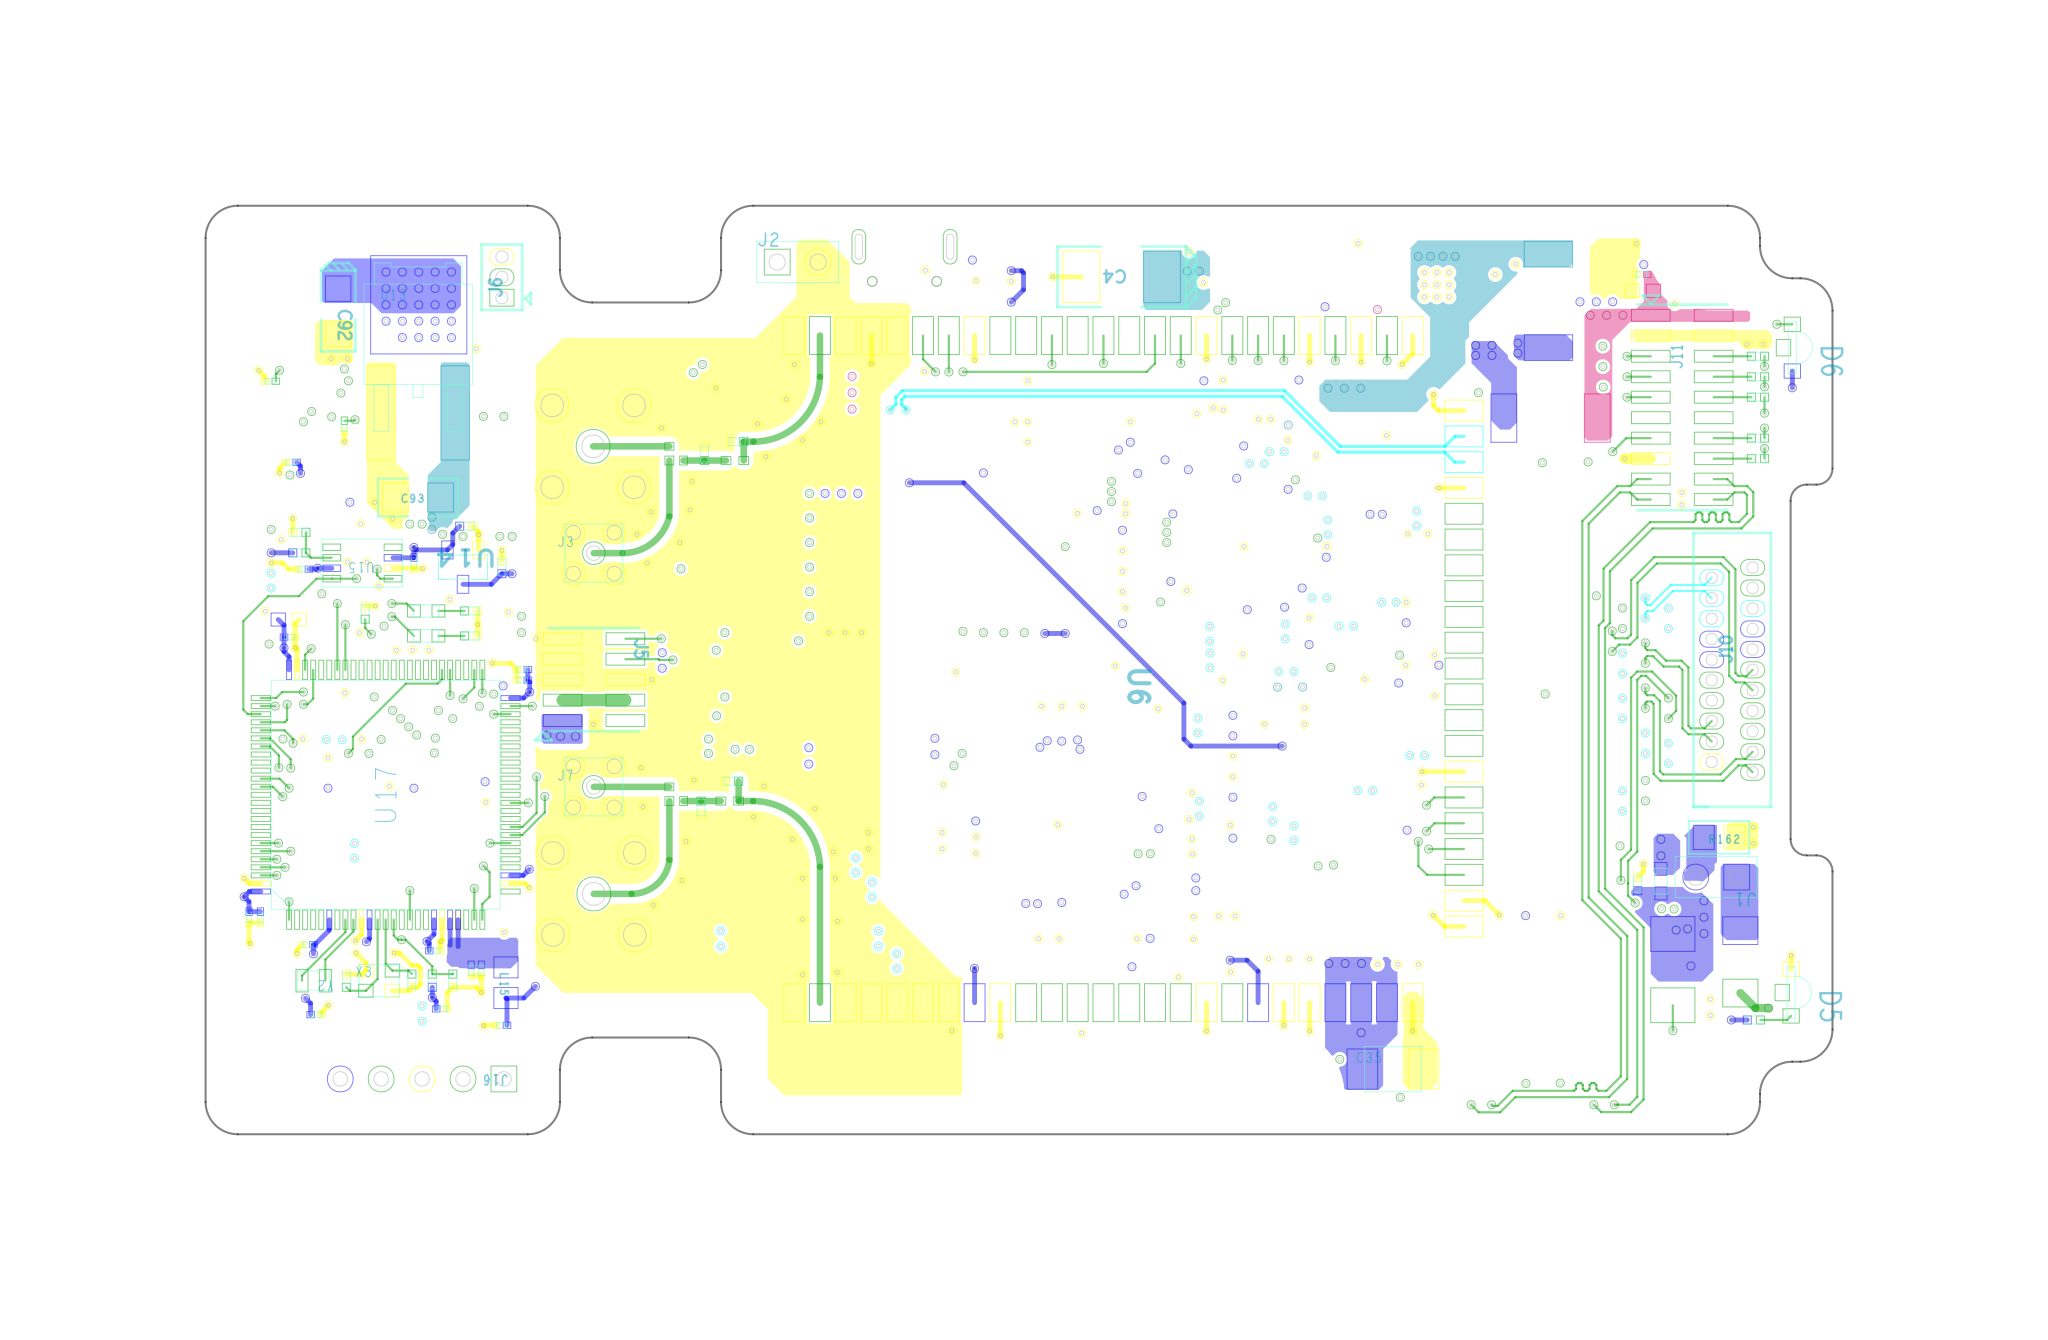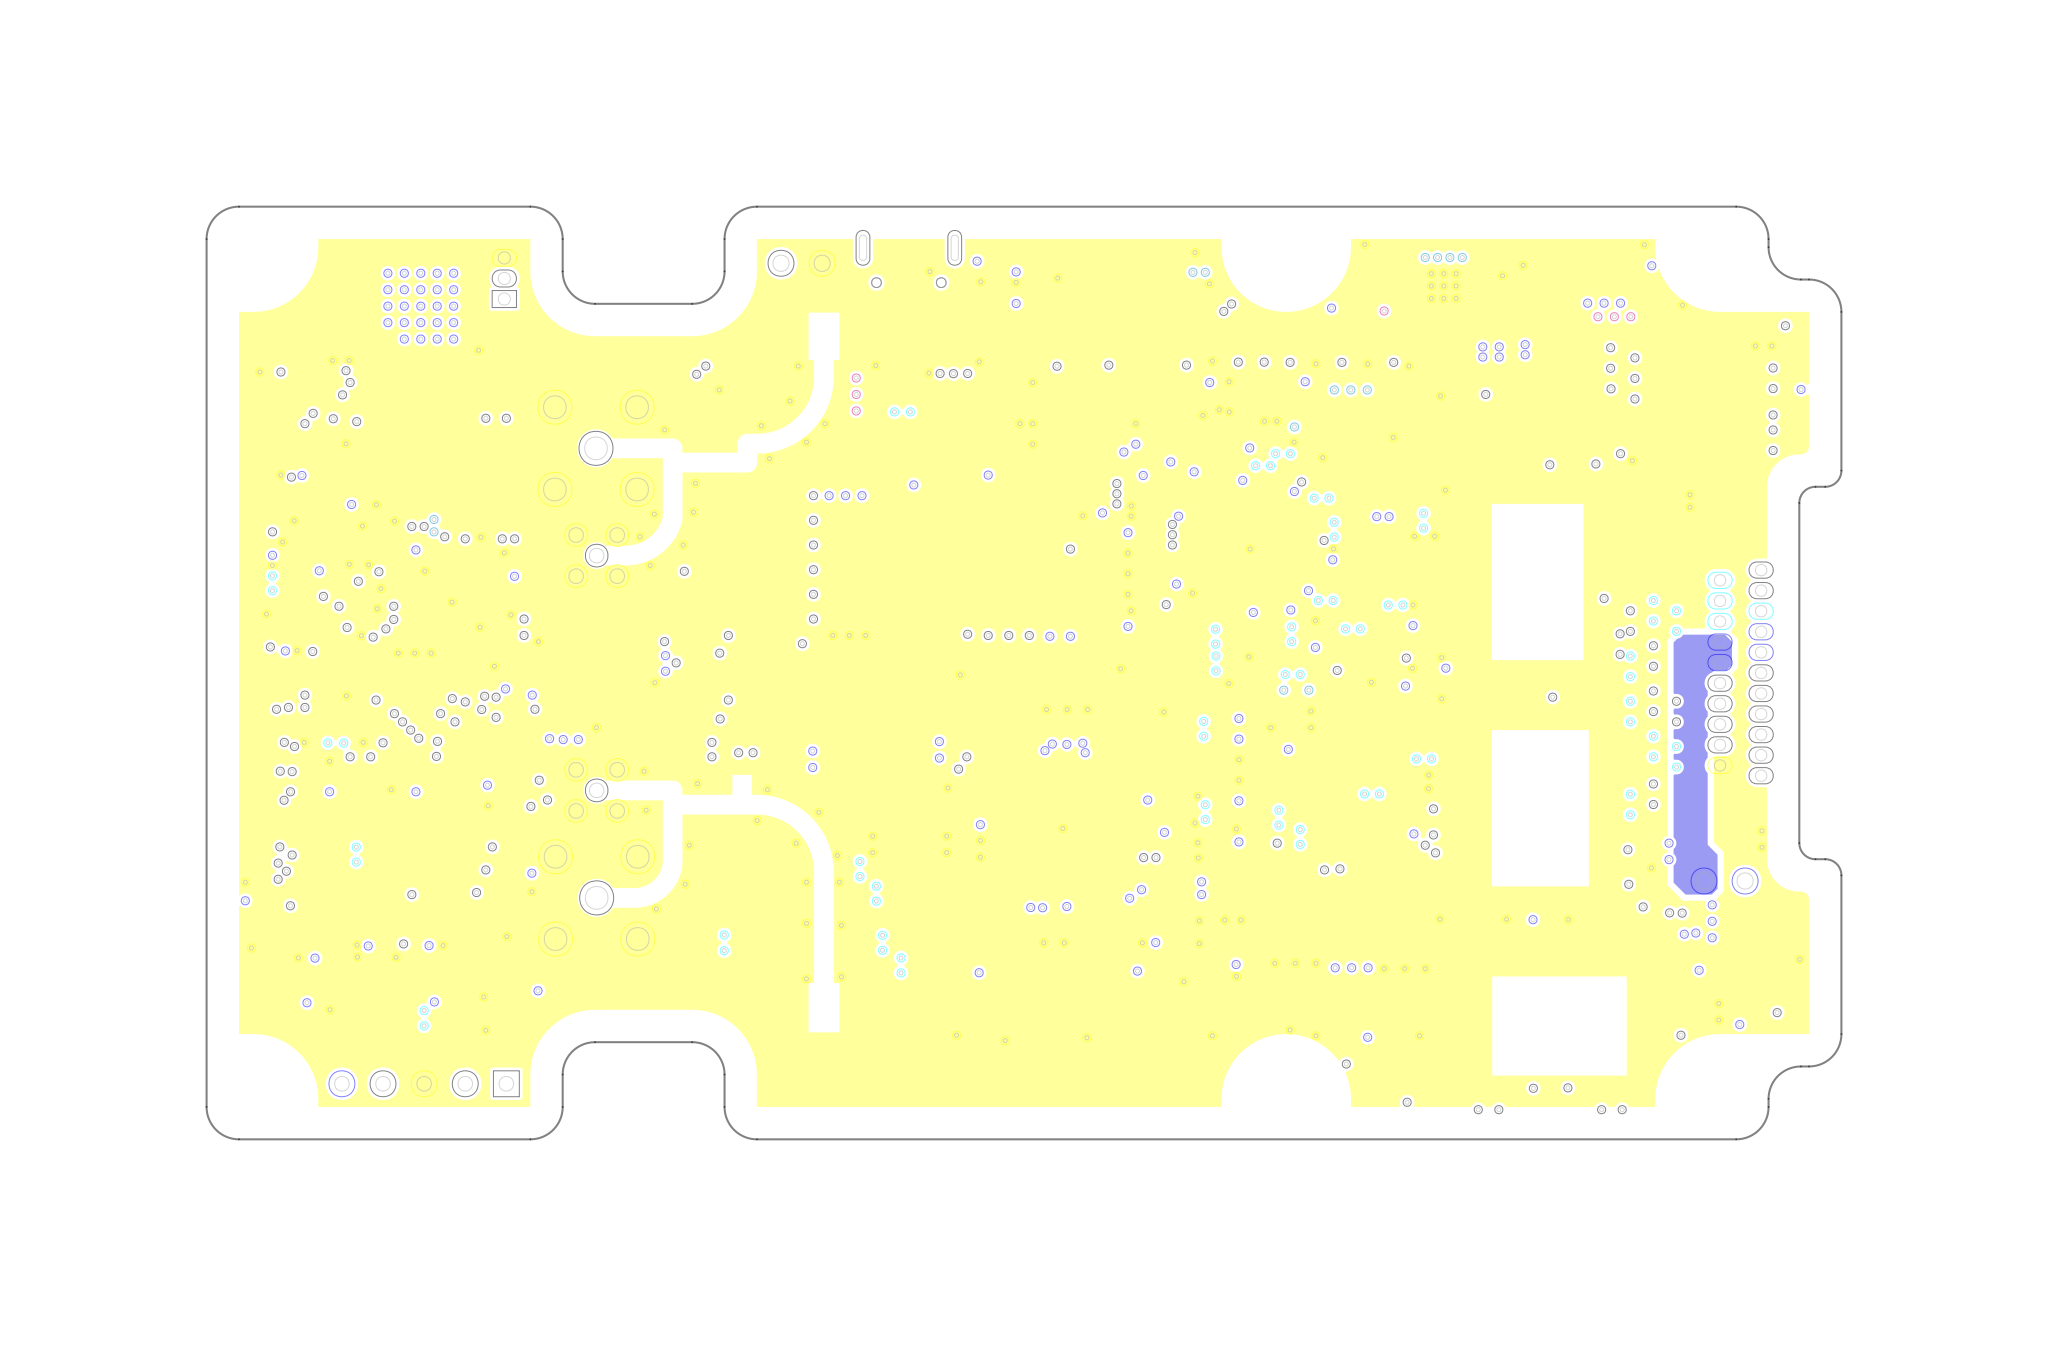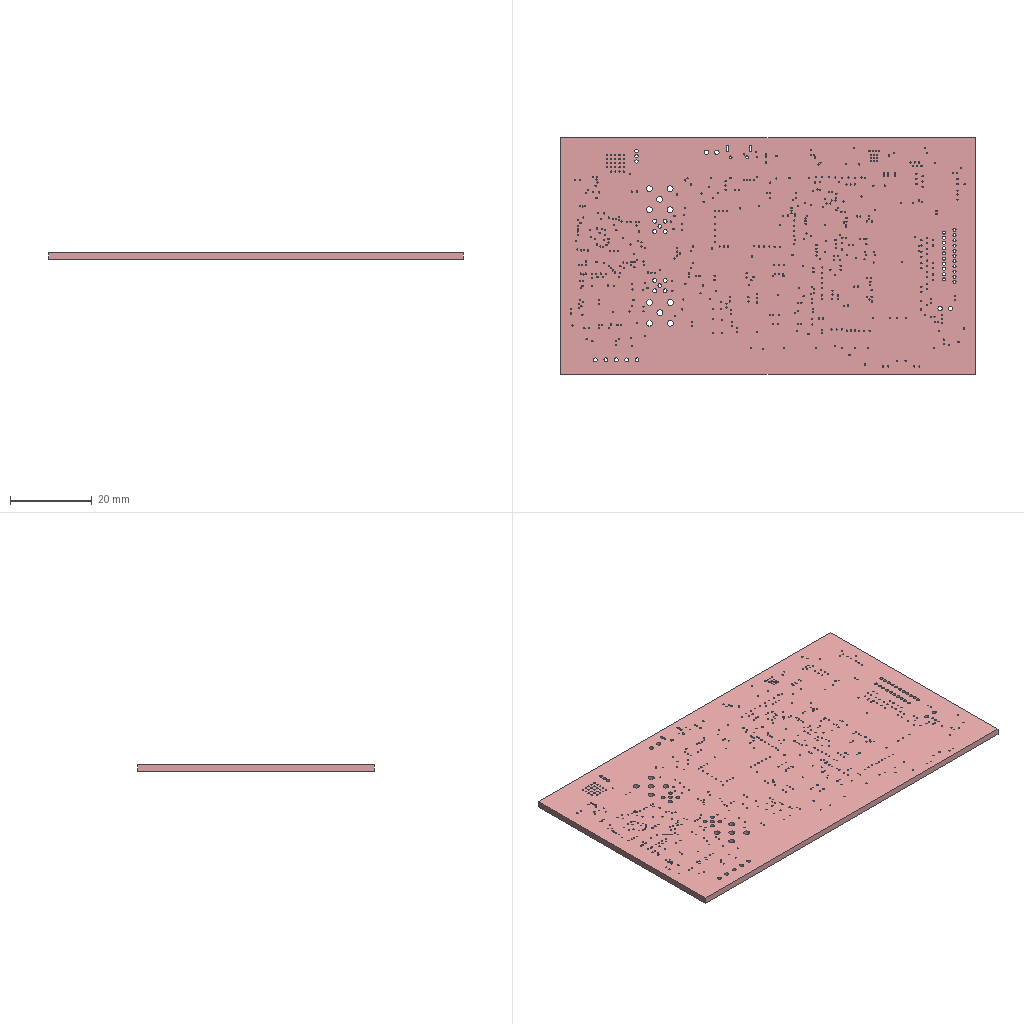Circuit board layout | Cadence Allegro | box 101.1 x 57.7 x 1.6 mm
Layer stack:
# Cadence Allegro layer stack of  (unit mm; from the constraint file cross-section; dielectric type: 0 not recorded (Allegro does not mark core vs prepreg), 3 surface material)
index,name,kind,layer,copper_thickness_mm,dielectric_type,dielectric_thickness_mm,dielectric_material,dielectric_constant
0,Top Surface,other,,,,,,
1,TOP,copper,TOP,0.0305,,,,
2,Dielectric1,dielectric,,,0,0.2032,FR-4,4.5
3,L2_GND,copper,L2_GND,0.0305,,,,
4,Dielectric2,dielectric,,,0,0.2032,FR-4,4.5
5,L3_S1,copper,L3_S1,0.0305,,,,
6,Dielectric3,dielectric,,,0,0.2032,FR-4,4.5
7,L4_PWR,copper,L4_PWR,0.0305,,,,
8,Dielectric4,dielectric,,,0,0.2032,FR-4,4.5
9,L5_GND,copper,L5_GND,0.0305,,,,
10,Dielectric5,dielectric,,,0,0.2032,FR-4,4.5
11,L6_S2,copper,L6_S2,0.0305,,,,
12,Dielectric6,dielectric,,,0,0.2032,FR-4,4.5
13,L7_GND,copper,L7_GND,0.0305,,,,
14,Dielectric7,dielectric,,,0,0.2032,FR-4,4.5
15,BOTTOM,copper,BOTTOM,0.0305,,,,
16,Bottom Surface,other,,,,,,
# drill layer pairs: low layer,high layer
drill_pair,TOP,BOTTOM
Part placement:
REFDES,COMP_VALUE,SYM_NAME,SYM_X,SYM_Y,SYM_ROTATE,SYM_MIRROR
C1,0.1uF,50V,0402C,3556.000,1461.000,270.000,NO
C2,4.7uF,50V,0805C,3075.000,2768.000,0.000,YES
C3,100uF,16V,C,CA45C,3630.000,2577.000,90.000,YES
C4,100uF,16V,C,CA45C,2295.000,2944.000,180.000,NO
C5,4.7uF,50V,0805C,2880.000,2411.000,0.000,YES
C6,4.7uF,50V,0805C,3649.000,1260.000,90.000,YES
C7,4.7uF,50V,0805C,3734.000,1260.000,90.000,YES
C8,4.7uF,50V,0805C,3507.000,2962.000,270.000,YES
C9,4.7uF,50V,0805C,3417.000,2962.000,270.000,YES
C10,0.1uF,50V,0402C,3338.000,2972.000,270.000,YES
C11,4.7uF,50V,0805C,3185.000,2527.000,270.000,YES
C12,4.7uF,50V,0805C,3270.000,2527.000,270.000,YES
C13,0.1uF,50V,0402C,3115.000,2552.000,270.000,YES
C14,0.1uF,50V,0402C,3249.000,3001.000,180.000,YES
C15,82pF,50V,0402C,2745.000,2582.000,0.000,YES
C16,22uF,10V,0603C,2704.000,1915.000,90.000,YES
C17,2.2uF,10V,0402C,2767.000,1928.000,90.000,YES
C18,82pF,50V,0402C,2889.000,2892.000,0.000,YES
C19,22uF,10V,0603C,2645.000,1914.000,90.000,YES
C20,0.1uF,50V,0402C,3658.000,1131.000,180.000,YES
C21,22uF,10V,0603C,2709.000,1220.000,270.000,YES
C22,22uF,10V,0603C,2654.000,1220.000,270.000,YES
C23,22uF,10V,0603C,2764.000,1220.000,270.000,YES
C24,22uF,10V,0603C,2599.000,1220.000,270.000,YES
C25,330uF,6.3V,C,CA45C,2734.000,1360.000,0.000,YES
C26,0.1uF,50V,0402C,3130.000,2632.000,180.000,YES
C27,0.1uF,10V,0402C,3019.000,2021.000,180.000,YES
C28,0.1uF,10V,0402C,2405.000,2980.000,0.000,YES
C29,0.1uF,10V,0402C,1980.000,2935.000,180.000,YES
C30,0.1uF,10V,0402C,2405.000,2880.000,0.000,YES
C31,0.1uF,10V(NC),0402C,2574.000,2688.000,270.000,YES
C32,0.1uF,10V,0402C,2405.000,2930.000,0.000,YES
C33,0.1uF,10V,0402C,2405.000,2830.000,0.000,YES
C34,0.1uF,10V,0402C,2904.000,1235.000,180.000,YES
C35,47uF,10V,B,CAKB,2958.000,1009.000,0.000,NO
C36,1pF,200V,0402C,1275.000,2511.492,90.000,NO
C37,1pF,200V,0402C,1355.000,2541.350,180.000,NO
C38,1pF,200V,0402C,1267.000,1647.547,270.000,NO
C39,1pF,200V,0402C,1342.512,1712.000,180.000,NO
C40,10pF,50V,0402C,2526.000,1923.000,180.000,YES
C41,10pF,50V,0402C,2526.000,1773.000,180.000,YES
C42,0.1uF,10V,0402C,2092.000,1371.000,90.000,YES
C43,0.1uF,10V,0402C,2099.000,1853.000,270.000,YES
C44,0.1uF,10V,0402C,2427.000,1326.000,180.000,YES
C45,0.1uF,10V,0402C,2199.000,1853.000,270.000,YES
C46,0.1uF,10V,0402C,1902.000,1595.000,90.000,YES
C47,10pF,50V,0402C,2526.000,1623.000,180.000,YES
C48,10pF,50V,0402C,2526.000,1723.000,180.000,YES
C49,1uF,25V,0402C,2427.000,1571.000,180.000,YES
C50,0.1uF,10V,0402C,2386.000,1224.000,180.000,YES
C51,0.1uF,10V,0402C,2332.000,1371.000,90.000,YES
C52,0.1uF,10V,0402C,2427.000,1684.000,180.000,YES
C53,27pF,50V,0402C,2197.000,1174.000,90.000,YES
C54,27pF,50V,0402C,1880.000,1173.000,90.000,YES
C55,1uF,25V,0402C,2142.000,1371.000,90.000,YES
C56,0.1uF,10V,0402C,2293.000,1275.000,270.000,YES
C57,0.1uF,10V,0402C,2149.000,1853.000,270.000,YES
C58,0.1uF,10V,0402C,2427.000,1521.000,180.000,YES
C59,0.1uF,10V,0402C,2427.000,1381.000,180.000,YES
C60,1uF,25V,0402C,2218.000,1356.000,180.000,YES
C61,0.1uF,10V,0402C,2218.000,1308.000,180.000,YES
C62,22pF,16V,0402C,2340.000,1889.000,180.000,YES
C63,22pF,16V,0402C,2340.000,2049.000,0.000,YES
C64,22uF,10V,0603C,2261.000,2303.000,270.000,YES
C65,0.1uF,25V,0201C,1859.000,1761.000,90.000,YES
C66,47uF,16V,C,CA45C,1759.000,1676.000,90.000,YES
C67,47uF,16V,C,CA45C,1470.000,2672.000,0.000,YES
C68,4.7uF,16V,0603C,3569.000,2910.000,0.000,NO
C69,0.1uF,25V,0201C,3566.000,2950.000,180.000,NO
C70,0.1uF,25V,0201C,3325.000,1364.000,90.000,YES
C71,0.1uF,25V,0201C,2819.000,2272.000,90.000,YES
C72,0.1uF,25V,0201C,2603.000,2090.000,270.000,YES
C73,0.1uF,25V,0201C,2736.000,2134.000,0.000,YES
C74,0.1uF,25V,0201C,2757.000,2433.000,0.000,YES
C77,0.1uF,25V,0201C,2659.000,2558.000,90.000,YES
C78,0.1uF,25V,0201C,2454.000,2573.000,90.000,YES
C79,4.7uF,16V,0603C,2574.000,2593.000,90.000,YES
C80,NC,0402C,2519.000,2583.000,90.000,YES
C81,0.1uF,25V,0201C,2629.000,2558.000,90.000,YES
C82,0.1uF,25V,0201C,2479.000,2573.000,90.000,YES
C83,0.022uF,25V,0402C,3384.000,1359.000,0.000,YES
C84,0.01uF,2KV,1812C,2975.000,1075.000,270.000,YES
C85,0.1uF,25V,0201C,2343.000,2365.000,0.000,YES
C86,0.1uF,25V,0201C,2343.000,2135.000,0.000,YES
C87,0.022uF,25V,0402C,3031.000,2149.000,0.000,YES
C88,0.01uF,2KV,1812C,2865.000,1715.000,0.000,YES
C89,0.1uF,25V,0201C,2343.000,2390.000,0.000,YES
C90,22uF,10V,0603C,2187.000,2422.000,270.000,YES
C91,47uF,16V,C,CA45C,1618.000,2240.000,90.000,YES
C92,10uF,16V,A,CA45A,380.000,2860.000,270.000,NO
C93,10uF,25V,1206C,575.000,2405.000,0.000,NO
C94,0.1uF,25V,0201C,565.000,2245.000,270.000,NO
C95,0.1uF,25V,0201C,295.000,2230.000,180.000,NO
C96,1uF,25V,0402C,780.000,2235.000,270.000,NO
C97,NC,0402C,437.000,1857.000,270.000,YES
C98,NC,0402C,293.000,1857.000,270.000,YES
C99,NC,0402C,257.000,2127.000,180.000,YES
C100,NC,0402C,257.000,2277.000,180.000,YES
C101,1uF,25V,0402C,693.000,2335.000,180.000,NO
C102,0.1uF,25V,0201C,715.000,2000.000,180.000,YES
C103,0.1uF,25V,0201C,446.000,2099.000,0.000,YES
C104,0.1uF,25V,0201C,430.000,1919.000,0.000,YES
C105,0.1uF,25V,0201C,956.000,2062.000,90.000,YES
C106,10uF,25V,1206C,1019.000,2040.000,270.000,YES
C107,22pF,16V,0402C,505.000,2205.000,90.000,YES
C108,0.1uF,25V,0201C,755.000,2125.000,180.000,YES
C109,10uF,25V,1206C,810.000,2200.000,0.000,YES
C110,22pF,16V,0402C,665.000,2205.000,270.000,YES
C111,0.1uF,25V,0201C,817.000,1476.000,90.000,YES
C112,2.2uF,25V,0603C,925.000,1896.000,0.000,YES
C113,2.2uF,25V,0603C,291.000,1997.000,180.000,YES
C114,22pF,16V,0402C,400.000,1225.000,90.000,NO
C115,4.7uF,16V,0603C,259.000,2107.000,180.000,NO
C116,0.1uF,25V,0201C,790.000,1476.000,90.000,YES
C117,0.1uF,25V,0201C,162.000,1380.000,270.000,NO
C118,0.1uF,25V,0201C,616.000,1298.000,0.000,NO
C119,0.1uF,25V,0201C,190.000,1380.000,270.000,NO
C120,0.1uF,25V,0201C,261.000,2064.000,0.000,NO
C121,0.1uF,25V,0201C,306.000,1313.000,180.000,NO
C122,0.1uF,25V,0201C,705.000,1250.000,270.000,NO
C123,0.1uF,25V,0201C,730.000,1250.000,270.000,NO
C124,22pF,16V,0402C,560.000,1225.000,270.000,NO
C125,0.1uF,25V,0201C,830.000,1959.000,180.000,NO
C126,0.1uF,25V,0201C,329.000,1730.000,270.000,YES
C127,0.1uF,25V,0201C,633.000,1156.000,0.000,NO
C128,0.1uF,25V,0201C,779.000,1116.000,180.000,NO
C129,0.1uF,25V,0201C,830.000,1985.000,180.000,NO
C130,0.1uF,25V,0201C,326.000,1142.000,0.000,NO
C131,0.1uF,25V,0201C,355.000,1730.000,270.000,YES
C132,1uF,25V,0402C,660.000,1225.000,90.000,NO
C133,0.1uF,25V,0201C,485.000,2795.000,0.000,YES
C134,0.1uF,25V,0201C,610.000,2740.000,180.000,YES
C135,0.1uF,25V,0201C,435.000,2380.000,270.000,YES
C136,0.1uF,25V,0201C,395.000,2579.000,90.000,NO
C137,0.1uF,25V,0201C,685.000,2755.000,90.000,YES
C138,0.1uF,25V,0201C,565.000,1730.000,90.000,YES
C139,0.1uF,25V,0201C,330.000,1195.000,90.000,YES
C140,0.1uF,25V,0201C,235.000,2785.000,180.000,YES
C141,0.1uF,25V,0201C,265.000,2491.000,0.000,NO
C142,0.1uF,25V,0201C,214.000,2689.000,0.000,NO
C143,0.1uF,25V,0201C,300.000,2785.000,180.000,YES
C144,0.1uF,25V,0201C,340.000,2730.000,90.000,YES
C145,0.022uF,25V,0402C,3044.000,1678.000,0.000,YES
C146,0.01uF,2KV,1812C,2660.000,1610.000,270.000,YES
D1,4A,30V,DO_214AA,3293.000,2785.000,270.000,YES
D2,4A,30V,DO_214AA,2946.000,2258.000,0.000,YES
D3,4A,30V,DO_214AA,3807.000,1271.000,270.000,NO
D4,5A,36V,DO_-214AA,3642.000,1252.000,90.000,NO
D5,S110GC-2A GRN,S110BC,3937.000,1196.000,270.000,NO
D6,S110BC-B4-1B BLUE,S110BC,3940.000,2771.000,270.000,NO
D7,LED-GREEN,0603L,1391.000,2115.000,180.000,YES
D8,LED-BLUE,0603L,1391.000,2175.000,180.000,YES
D9,LED-BLUE,0603L,1391.000,2235.000,180.000,YES
D10,LED-BLUE,0603L,1391.000,2295.000,180.000,YES
D11,LED-BLUE,0603L,1391.000,2355.000,180.000,YES
D12,LED-BLUE,0603L,1391.000,2415.000,180.000,YES
D13,LED-BLUE,0603L,595.000,2128.000,0.000,NO
D14,LED-GREEN,0603L,595.000,2067.000,0.000,NO
F1,2.5A,32V,1206,3862.000,1258.000,270.000,YES
F2,5A,32V,SF-1206F500,1494.000,2899.000,180.000,YES
J1,1*2P-2.54mm_ZZ(NC),2P54-1-2,3748.000,1478.000,180.000,NO
J2,1*2P-2.54mm_ZZ(NC),2P54-1-2,1503.000,2980.000,0.000,NO
J3,MMCX-KHD2,MMCX-KHD2,1004.662,2269.205,0.000,NO
J4,DOSIN-806-0331,DOSIN-806-0331,1003.000,2530.000,270.000,NO
J5,HX2*5P-1.27mm-ZK,1P27-2-5-L-SMT,1005.090,1960.180,270.000,NO
J6,1*3Pin_1.27mm_ZZ,1P27-1-3,780.000,2893.000,90.000,NO
J7,MMCX-KHD2,MMCX-KHD2,1004.662,1698.339,0.000,NO
J8,DOSIN-806-0331,DOSIN-806-0331,1004.662,1437.000,0.000,NO
J9,MK5P-ZK,MICRO-USB_5_9,1764.000,2897.468,180.000,YES
J10,J30J-21TJW-J,J30J-21TJW-J,3787.000,1984.000,90.000,NO
J11,1P27m1P0-2m10P_SMT_NC,1P27-2-10-L-SMT,3665.000,2625.000,90.000,NO
J16,1*5Pin_2.54mm_ZZ,SIP-5-2R5,785.000,985.000,180.000,NO
L1,15nH,2.1A,0603L,3613.000,1468.000,90.000,NO
L2,22uH,2.3A,WHC,-5504.000,-1973.000,0.000,NO
L3,15uH,2.6A,WHC,7910.000,-5962.000,90.000,NO
L4,1.5uH,9.1A,0603L,2894.000,1831.000,0.000,YES
L5,15nH,2.1A,0603L,3362.000,2520.000,90.000,YES
L6,3.9nH,0402L,1349.488,2495.350,180.000,NO
L7,3.9nH,0402L,1337.000,1663.689,180.000,NO
L8,ICMEF212P900MFR,ICT_ICMEF212P900MFR_S,1750.000,2755.000,0.000,YES
L9,1.3A,120Ohms,0402L,2386.000,1279.000,180.000,YES
L10,1.3A,120Ohms,0402L,2427.000,1476.000,180.000,YES
L11,1.3A,120Ohms,0402L,2427.000,1431.000,180.000,YES
L12,1.3A,120Ohms,0402L,2224.000,1259.000,180.000,YES
L13,330Ohms,1.5A,0805L,1608.000,1775.000,0.000,YES
L14,1.5A,330Ohms,0805L,1117.000,2046.000,270.000,YES
L15,1.5A,330Ohms,0805L,790.000,1220.000,270.000,NO
Q1,L14C1/TO,SOT-323,3755.000,2815.000,270.000,YES
R1,100k,1%,0402R,3249.000,2942.000,180.000,YES
R2,100k,1%,0402R,2889.000,2947.000,180.000,YES
R3,100k,1%,0402R,3130.000,2682.000,180.000,YES
R4,100k,1%,0402R,2745.000,2632.000,180.000,YES
R5,11k,1%,0402R,2889.000,3001.000,180.000,YES
R6,31.6k,1%,0402R,2745.000,2532.000,180.000,YES
R7,1.02M,1%,0402R,3019.000,1971.000,180.000,YES
R8,200R,1%,0402R,3840.000,1129.000,180.000,NO
R9,1M,1%,0402R,2769.000,2021.000,180.000,YES
R10,147k,1%,0402R,3019.000,1921.000,0.000,YES
R11,200R,0402R,3845.000,2820.000,90.000,YES
R12,10k,0402R,1807.000,2423.000,270.000,YES
R13,1K,0402R,1873.098,1935.000,180.000,YES
R14,0R,0402R,1980.000,2985.000,180.000,YES
R15,10k,0402R,1957.000,2423.000,270.000,YES
R16,0R,0402R,1980.000,2855.000,180.000,YES
R17,0R,0402R,2007.000,2423.000,90.000,YES
R18,0R,0402R,1980.000,2805.000,180.000,YES
R19,4.7K,0402R,3665.000,2815.000,270.000,YES
R20,100R,0402R,2634.000,2780.000,270.000,YES
R21,0R,0402R,2057.000,2423.000,90.000,YES
R22,4.7K,0402R,3615.000,2815.000,90.000,YES
R23,100R,0402R,2684.000,2780.000,270.000,YES
R24,75R,0402R,1900.000,2805.000,180.000,YES
R25,75R,0402R,1900.000,2855.000,180.000,YES
R26,49.9R,0402R,2526.000,1873.000,0.000,YES
R27,49.9R,0402R,2526.000,1823.000,0.000,YES
R28,49.9R,0402R,2526.000,1673.000,0.000,YES
R29,49.9R,0402R,2526.000,1573.000,0.000,YES
R30,12k,0402R,2427.000,1619.000,180.000,YES
R31,12k,0402R,2282.000,1371.000,90.000,YES
R32,10k(NC),0402R,1813.000,2774.000,90.000,YES
R33,10k(NC),0402R,1684.000,2774.000,90.000,YES
R34,0R,0402R,2042.000,1371.000,270.000,YES
R39,0R,NC,0402R,3535.000,1940.000,0.000,YES
R40,0R,NC,0402R,3535.000,2110.000,0.000,YES
R41,0R,0402R,3615.000,1890.000,180.000,YES
R42,0R,0402R,3615.000,2160.000,180.000,YES
R44,0R,NC,0402R,3535.000,1890.000,0.000,YES
R45,0R,NC,0402R,3535.000,2160.000,0.000,YES
R46,0R,0402R,3615.000,1940.000,180.000,YES
R47,0R,0402R,3615.000,2110.000,180.000,YES
R49,0R,NC,0402R,3479.000,2492.000,180.000,YES
R50,0R,NC,0402R,3850.000,2550.000,180.000,NO
R51,0R,NC,0402R,3535.000,2050.000,0.000,YES
R52,0R,0402R,2554.000,2508.000,180.000,YES
R53,0R,NC,0402R,3535.000,2000.000,0.000,YES
R54,0R,0402R,3850.000,2500.000,180.000,NO
R55,0R,0402R,2474.000,2508.000,0.000,YES
R56,0R,NC,0402R,3266.000,1359.000,0.000,YES
R57,0R,0402R,3615.000,2050.000,180.000,YES
R58,0R,0402R,3615.000,2000.000,180.000,YES
R59,75R,0402R,2868.000,994.000,90.000,YES
R60,6.19K,0603R,2745.000,2479.000,180.000,YES
R61,0R,NC,0805R,3761.000,1575.000,180.000,YES
R62,0R,NC,0805R,2490.000,1150.000,180.000,YES
R63,NC,4.7K,0402R,2338.000,2325.000,180.000,YES
R64,4.7K,0402R,2455.000,2690.000,180.000,YES
R65,470K,0402R,2338.000,2097.000,180.000,YES
R66,0R,NC,0402R,3031.000,2099.000,180.000,YES
R67,NC,4.7K,0402R,2338.000,2175.000,180.000,YES
R68,75R,0402R,3509.000,2263.000,90.000,YES
R69,0R,0402R,2338.000,2225.000,180.000,YES
R70,NC,4.7K,0402R,2338.000,2275.000,180.000,YES
R71,270R,0402R,1491.000,2115.000,180.000,YES
R73,270R,0402R,1491.000,2175.000,180.000,YES
R75,270R,0402R,1491.000,2235.000,180.000,YES
R77,270R,0402R,1491.000,2295.000,180.000,YES
R79,0R,0402R,2235.000,2421.000,270.000,YES
R80,270R,0402R,1491.000,2355.000,180.000,YES
R82,270R,0402R,1491.000,2415.000,180.000,YES
R84,0R,NC,0805R,1417.500,1932.000,0.000,YES
R85,0R,NC,0805R,1417.500,2032.000,0.000,YES
R86,49.9R,0402R,485.000,1857.000,270.000,YES
R87,49.9R,0402R,245.000,1857.000,270.000,YES
R88,0R,0402R,257.000,2177.000,0.000,YES
R89,4.7K,NC,0402R,285.000,2320.000,0.000,NO
R90,49.9R,0402R,257.000,2077.000,180.000,YES
R91,49.9R,0402R,257.000,2327.000,180.000,YES
R92,0R,0402R,389.000,1857.000,90.000,YES
R93,0R,0402R,341.000,1857.000,90.000,YES
R94,0R,0402R,257.000,2227.000,0.000,YES
R95,4.7K,0402R,285.000,2270.000,0.000,NO
R96,4.7K,0402R,450.000,2205.000,90.000,YES
R97,4.7K,0402R,400.000,2205.000,90.000,YES
R98,12K,0402R,446.000,2124.000,90.000,NO
R99,270R,0402R,705.000,2128.000,0.000,NO
R100,270R,0402R,705.000,2067.000,0.000,NO
R101,4.7K,0402R,610.000,1225.000,270.000,NO
R102,0R,NC,0402R,405.000,1735.000,90.000,YES
R103,0R,NC,0402R,455.000,1735.000,90.000,YES
R104,0R,0402R,635.000,2355.000,270.000,YES
R105,0R,0402R,685.000,2355.000,270.000,YES
R106,0R,0402R,760.000,2370.000,270.000,YES
R111,0R,0402R,815.000,2370.000,270.000,YES
R112,120R,0805R,795.000,1165.000,90.000,YES
R113,0R,NC,0402R,615.000,1740.000,90.000,YES
R114,0R,NC,0402R,665.000,1740.000,90.000,YES
R115,100k,0402R,181.000,1340.000,180.000,YES
R116,4.7K,0402R,770.000,1265.000,0.000,YES
R142,0R,NC,0402R,3535.000,1664.000,0.000,YES
R143,0R,NC,0402R,3535.000,1714.000,0.000,YES
R144,0R,0402R,3615.000,1664.000,180.000,YES
R145,0R,0402R,3615.000,1714.000,180.000,YES
R146,0R,0402R,3535.000,1830.000,0.000,YES
R147,0R,0402R,3535.000,1780.000,0.000,YES
R148,0R,NC,0402R,3615.000,1830.000,180.000,YES
R149,0R,NC,0402R,3615.000,1780.000,180.000,YES
R150,0R,NC,0402R,3044.000,1628.000,180.000,YES
R151,75R,0402R,3529.000,1580.000,0.000,YES
R152,0R,NC,0402R,3487.000,2750.000,180.000,YES
R153,0R,NC,0402R,3850.000,2750.000,180.000,NO
R154,0R,NC,0402R,3487.000,2700.000,180.000,YES
R155,0R,NC,0402R,3850.000,2700.000,180.000,NO
R156,0R,NC,0402R,3488.000,2650.000,180.000,YES
R157,0R,NC,0402R,3850.000,2650.000,180.000,NO
R158,200R,0402R,1857.000,2423.000,90.000,YES
R159,4.7K,NC,0402R,181.000,1390.000,180.000,YES
R160,4.7K,NC,0402R,786.000,1711.000,0.000,YES
R161,100k,0402R,786.000,1661.000,180.000,YES
R162,0R,0805R,3755.000,1575.000,0.000,NO
RR1,0R,04022R,1189.370,1663.689,90.000,NO
RR2,0R,04022R,1189.370,2495.350,90.000,NO
U1,RT8279GSP,SOP8,2970.010,2849.606,180.000,YES
U2,RT8279GSP,SOP8,2847.010,2481.606,180.000,YES
U3,TPS63020DSJT,DSJ14_2P85X1P58,2889.000,1961.000,90.000,YES
U4,SW-8,KE_BMKG,2032.000,2182.000,180.000,YES
U5,MAX3221EEAE,SSOP16,2195.000,2895.000,90.000,YES
U6,CX660X,LC6500_PAD_S,2313.000,1986.000,270.000,NO
U7,LAN9730i_ABZJ,SMSC_QFN_56_S,2138.455,1606.000,90.000,YES
U9,IP175GI,QFN_48,2594.000,2285.000,90.000,YES
U10,HX0068ANL,HX0068ANL,3324.000,1132.000,90.000,YES
U11,AT24C01-10SI-2.7,SOIC8_300_206,2239.000,2712.000,180.000,YES
U12,HX0068ANL,HX0068ANL,3282.000,2204.000,180.000,YES
U13,AMS1117-3.3,1A,TO252AA,485.000,2613.000,0.000,NO
U14,65K5,SOT23-28X44,685.000,2235.000,180.000,NO
U15,TXS0102DCT,SSOP8-TXS0102DCT,513.910,2206.720,180.000,NO
U16,LAN8720A,QFN24,562.000,1992.000,180.000,YES
U17,STM32F407VGT6,LQFP100-14X14MM,496.000,1679.000,90.000,NO
U18,MAX3077EESA,SO8-25X75,430.000,1510.000,180.000,YES
U19,MAX3232ESE,SOIC16,610.000,2565.000,180.000,YES
U20,MAX3051ESA,SO8-25X75,540.000,1190.000,270.000,YES
U21,MAX3077EESA,SO8-25X75,640.000,1509.000,180.000,YES
U22,MAX3221EEAE,SSOP16,275.000,2540.000,180.000,YES
U23,HX0068ANL,HX0068ANL,3286.000,1655.000,180.000,YES
X1,ABM10-25.000MHZ-8pF-R50-4-D30,ABM10-2_5X2_0-0_55,2338.000,1969.000,270.000,YES
X2,ABM10-25.000MHZ-8pF-R50-4-D30,ABM10-2_5X2_0-0_55,585.000,2205.000,0.000,YES
X3,ABM10-25.000MHZ-8pF-R50-4-D30,ABM10-2_5X2_0-0_55,480.000,1225.000,0.000,NO
Y1,25MHz,27pF,ABM7-25MHZ,2043.000,1188.000,180.000,YES
Y2,32.768K,ABS06,320.000,1225.000,180.000,NO
Pad and via stacks, first 107 of 133 lines:
# Allegro (Cadence) via spans and padstacks; design units: ("mils" 3 1000)
# via spans: padstack,start_layer,end_layer,net_example,count
VIA_20D10,ETCH/TOP,ETCH/BOTTOM,3V3,618
# Allegro padstack definitions: name,start_layer,end_layer,drill,plating,holeType,type
SMDX0_5_Y0_5,"ETCH/TOP","ETCH/TOP",0.0,"PLATED","none","smd"
SMDX0_3_Y0_3,"ETCH/TOP","ETCH/TOP",0.0,"PLATED","none","smd"
SMDX0_8_Y0_76,"ETCH/TOP","ETCH/TOP",0.0,"PLATED","none","smd"
SMDX1_25_Y1_0,"ETCH/TOP","ETCH/TOP",0.0,"PLATED","none","smd"
SMDX3_4_Y1_3,"ETCH/TOP","ETCH/TOP",0.0,"PLATED","none","smd"
SMDX1_6_Y1_2,"ETCH/TOP","ETCH/TOP",0.0,"PLATED","none","smd"
SMDX2_5_Y1_9,"ETCH/TOP","ETCH/TOP",0.0,"PLATED","none","smd"
SMDX2_5_Y2_3,"ETCH/TOP","ETCH/TOP",0.0,"PLATED","none","smd"
SMDX2_8_Y1_5,"ETCH/TOP","ETCH/TOP",0.0,"PLATED","none","smd"
SMDX2_5_Y0_76,"ETCH/TOP","ETCH/TOP",0.0,"PLATED","none","smd"
SMDX4_Y2_35,"ETCH/TOP","ETCH/TOP",0.0,"PLATED","none","smd"
SMDX3_2_Y3_2,"ETCH/TOP","ETCH/TOP",0.0,"PLATED","none","smd"
SMDX2_5_Y1_5,"ETCH/TOP","ETCH/TOP",0.0,"PLATED","none","smd"
SMDX0_5_Y0_34,"ETCH/TOP","ETCH/TOP",0.0,"PLATED","none","smd"
SMDX0_9_Y0_7,"ETCH/TOP","ETCH/TOP",0.0,"PLATED","none","smd"
CIRX1_8_Y0_6,"ETCH/TOP","ETCH/TOP",0.0,"PLATED","none","smd"
SMDX2_2_Y0_64,"ETCH/TOP","ETCH/TOP",0.0,"PLATED","none","smd"
SMDX2_3_Y2_3,"ETCH/TOP","ETCH/TOP",0.0,"PLATED","none","smd"
CIRX1_1_Y0_4,"ETCH/TOP","ETCH/TOP",0.0,"PLATED","none","smd"
SMDX1_1_Y0_4,"ETCH/TOP","ETCH/TOP",0.0,"PLATED","none","smd"
CIRX1_8_Y0_3,"ETCH/TOP","ETCH/TOP",0.0,"PLATED","none","smd"
SMDX6_7_Y6_7,"ETCH/TOP","ETCH/TOP",0.0,"PLATED","none","smd"
SMDX3_0_Y1_6,"ETCH/TOP","ETCH/TOP",0.0,"PLATED","none","smd"
CIRX1_4_Y0_36,"ETCH/TOP","ETCH/TOP",0.0,"PLATED","none","smd"
CIRX0_6_Y0_24,"ETCH/TOP","ETCH/TOP",0.0,"PLATED","none","smd"
SMDSP_TPS63020,"ETCH/TOP","ETCH/TOP",0.0,"PLATED","none","smd"
SMDX5_9_Y5_9,"ETCH/TOP","ETCH/TOP",0.0,"PLATED","none","smd"
SMDX4_0_Y4_0,"ETCH/TOP","ETCH/TOP",0.0,"PLATED","none","smd"
CIRX1_0_Y0_24,"ETCH/TOP","ETCH/TOP",0.0,"PLATED","none","smd"
SMDX1_0_Y0_24,"ETCH/TOP","ETCH/TOP",0.0,"PLATED","none","smd"
SMDX1_4_Y1_0,"ETCH/TOP","ETCH/TOP",0.0,"PLATED","none","smd"
SMDX1_4_Y0_75,"ETCH/TOP","ETCH/TOP",0.0,"PLATED","none","smd"
18P5X15REC,"ETCH/TOP","ETCH/TOP",0.0,"PLATED","none","smd"
SMD1R90X3R40,"ETCH/TOP","ETCH/TOP",0.0,"PLATED","none","smd"
25RD,"ETCH/TOP","ETCH/TOP",0.0,"PLATED","none","smd"
SMD0R89X0R81,"ETCH/TOP","ETCH/TOP",0.0,"PLATED","none","smd"
SMD2D8X2D0RT,"ETCH/TOP","ETCH/TOP",0.0,"PLATED","none","smd"
SMD0R60X0R50,"ETCH/TOP","ETCH/TOP",0.0,"PLATED","none","smd"
28X44REC,"ETCH/TOP","ETCH/TOP",0.0,"PLATED","none","smd"
RX47Y12D0T,"ETCH/TOP","ETCH/TOP",0.0,"NON_PLATED","none","smd"
25X75OV,"ETCH/TOP","ETCH/TOP",0.0,"PLATED","none","smd"
R90X126,"ETCH/TOP","ETCH/TOP",0.0,"NON_PLATED","none","smd"
SMDOBL8X34,"ETCH/TOP","ETCH/TOP",0.0,"PLATED","none","smd"
SMDSQU150,"ETCH/TOP","ETCH/TOP",0.0,"PLATED","none","smd"
090X080,"ETCH/TOP","ETCH/TOP",0.0,"PLATED","none","smd"
R1_1X1_4,"ETCH/TOP","ETCH/TOP",0.0,"NON_PLATED","none","smd"
SMD1R60X1R80,"ETCH/TOP","ETCH/TOP",0.0,"PLATED","none","smd"
SMD1R30X1R50,"ETCH/TOP","ETCH/TOP",0.0,"PLATED","none","smd"
PAD32,"ETCH/TOP","ETCH/TOP",0.0,"PLATED","none","smd"
SMD1_45X1_8,"ETCH/TOP","ETCH/TOP",0.0,"PLATED","none","smd"
PAD31,"ETCH/TOP","ETCH/TOP",0.0,"PLATED","none","smd"
PAD30,"ETCH/TOP","ETCH/TOP",0.0,"PLATED","none","smd"
P2_18C1_72,"ETCH/TOP","ETCH/TOP",0.0,"PLATED","none","smd"
PAD29,"ETCH/TOP","ETCH/TOP",0.0,"PLATED","none","smd"
PAD25,"ETCH/TOP","ETCH/TOP",0.0,"NON_PLATED","none","smd"
PAD24,"ETCH/TOP","ETCH/TOP",0.0,"NON_PLATED","none","smd"
PAD7,"ETCH/TOP","ETCH/TOP",0.0,"PLATED","none","smd"
RECTANGLE60X50,"ETCH/TOP","ETCH/TOP",0.0,"PLATED","none","smd"
PAD11,"ETCH/TOP","ETCH/TOP",0.0,"PLATED","none","smd"
SMDX2_1_Y0_76,"ETCH/TOP","ETCH/TOP",0.0,"PLATED","none","smd"
SMDX2_6_Y2_2,"ETCH/TOP","ETCH/TOP",0.0,"PLATED","none","smd"
R250_230,"ETCH/TOP","ETCH/TOP",0.0,"PLATED","none","smd"
R2_54C2_65,"ETCH/TOP","ETCH/TOP",0.0,"PLATED","none","smd"
PAD33,"ETCH/TOP","ETCH/TOP",0.0,"PLATED","none","smd"
SMDX5_0_Y1_2,"ETCH/TOP","ETCH/TOP",0.0,"PLATED","none","smd"
SMDX5_0_Y1_2B,"ETCH/BOTTOM","ETCH/BOTTOM",0.0,"PLATED","none","smd"
SMDX1_4_Y0_4,"ETCH/TOP","ETCH/TOP",0.0,"PLATED","none","smd"
S1_5C2_4,"ETCH/TOP","ETCH/TOP",0.0,"PLATED","none","smd"
R1_7X2_0,"ETCH/TOP","ETCH/TOP",0.0,"PLATED","none","smd"
P2_159C2_743,"ETCH/TOP","ETCH/TOP",0.0,"PLATED","none","smd"
R72X28,"ETCH/TOP","ETCH/TOP",0.0,"NON_PLATED","none","smd"
CIRX2_2_Y0_6,"ETCH/TOP","ETCH/TOP",0.0,"PLATED","none","smd"
SMD0R60X2R20,"ETCH/TOP","ETCH/TOP",0.0,"PLATED","none","smd"
SMD2R5X2R5MM,"ETCH/TOP","ETCH/TOP",0.0,"NON_PLATED","none","smd"
SMD0R3X1MM,"ETCH/TOP","ETCH/TOP",0.0,"NON_PLATED","none","smd"
SMD1X0R3MM,"ETCH/TOP","ETCH/TOP",0.0,"NON_PLATED","none","smd"
SMDX2_5_Y2_5,"ETCH/TOP","ETCH/TOP",0.0,"PLATED","none","smd"
CIRX0_8_Y0_28,"ETCH/TOP","ETCH/TOP",0.0,"PLATED","none","smd"
SMD50_25,"ETCH/TOP","ETCH/TOP",0.0,"NON_PLATED","none","smd"
SMDX0_9_Y0_8,"ETCH/TOP","ETCH/TOP",0.0,"PLATED","none","smd"
SMDX2_6_Y2_0,"ETCH/TOP","ETCH/TOP",0.0,"PLATED","none","smd"
PAD35,"ETCH/TOP","ETCH/TOP",0.0,"PLATED","none","smd"
PAD36,"ETCH/TOP","ETCH/TOP",0.0,"NON_PLATED","none","smd"
SMD240_235,"ETCH/TOP","ETCH/TOP",0.0,"PLATED","none","smd"
S62,"ETCH/TOP","ETCH/TOP",0.0,"PLATED","none","smd"
SMD63X48,"ETCH/TOP","ETCH/TOP",0.0,"PLATED","none","smd"
R1_1X0_4,"ETCH/TOP","ETCH/TOP",0.0,"PLATED","none","smd"
SMD70_230,"ETCH/TOP","ETCH/TOP",0.0,"PLATED","none","smd"
R2_3X2_3,"ETCH/TOP","ETCH/TOP",0.0,"PLATED","none","smd"
R1_77X0_51,"ETCH/TOP","ETCH/TOP",0.0,"PLATED","none","smd"
SMD_R512X925P0S40,"ETCH/TOP","ETCH/TOP",0.0,"PLATED","none","smd"
PAD44,"ETCH/TOP","ETCH/TOP",0.0,"NON_PLATED","none","smd"
PAD43,"ETCH/TOP","ETCH/TOP",0.0,"PLATED","none","smd"
SMDX1_5_Y1_0,"ETCH/TOP","ETCH/TOP",0.0,"PLATED","none","smd"
SMD35_40,"ETCH/TOP","ETCH/TOP",0.0,"PLATED","none","smd"
R2_4X0_74,"ETCH/TOP","ETCH/TOP",0.0,"PLATED","none","smd"
SMD1_6R3_0,"ETCH/TOP","ETCH/TOP",0.0,"PLATED","none","smd"
THC3R0_1R35,"ETCH/TOP","ETCH/BOTTOM",53.15,"PLATED","circle_drill","through"
THC6R0_2R7,"ETCH/TOP","ETCH/BOTTOM",106.299,"PLATED","circle_drill","through"
MER3R5_3R5,"ETCH/TOP","ETCH/BOTTOM",137.795,"NON_PLATED","circle_drill","through"
THR1R0_0R7,"ETCH/TOP","ETCH/BOTTOM",27.559,"PLATED","circle_drill","through"
THS1R0_0R7,"ETCH/TOP","ETCH/BOTTOM",27.559,"PLATED","circle_drill","through"
THS1R6_1R0,"ETCH/TOP","ETCH/BOTTOM",39.37,"PLATED","circle_drill","through"
Design rules, without the lines most boards share, first 12 of 61 lines:
# Cadence Allegro design rules of  (from the Constraint Manager export constraints.dcfx, design unit mil; typed fields in mm)
# columns: name | kind | enabled | priority | scope1 | scope2 | descriptor | typed fields (field=value)
# Allegro precedence (priority 1 wins): 1 Region class-to-class, 2 Region class, 3 Region, 4 class-to-class, 5 DiffPair/Bus/NetGroup override, 6 NetClass, 7 constraint set (CSet) default
# per-layer values are written LAYER=value in the descriptor and LAYER:mm in the typed field; a maximum of 0 means no limit set
# --- net classes (and buses / net groups) ---
RF | NetClass | enabled | 6 | N17786541, N16899432, N16898912, N16897265, N173979642, N17770006, N16900333, N16900328 | All | Net Class (SpacingCSet=RF) (members: 8 Net) | spacingcset=RF
DIFF75 | NetClass | enabled | 6 | DIFF75_2, DIFF75_1 | All | Net Class (PhysicalCSet=DIFF75OHM) (members: 2 DiffPair) overrides: (DIFFP_PHASE_TOL=5 mil) | physicalcset=DIFF75OHM diffp_phase_tol=5mil
DIFF100 | NetClass | enabled | 6 | CAN1, DIFF100_1, DIFF100_2, DIFF100_3, DIFF100_4, DIFF100_5, ETH_RX, ETH_TX, LAN_R0, LAN_R1, LAN_R2, LAN_R4, LAN_T0, LAN_T1, LAN_T2, LAN_T4, RS422_R1, RS422_R2, RS422_T1, RS422_T2, RXI0, RXI1, RXI2, TXO0, TXO1, TXO2, DIFF100_6, DIFF100_7 | All | Net Class (PhysicalCSet=DIFF100OHM) (members: 28 DiffPair) overrides: (DIFFP_PHASE_TOL=5 mil) | physicalcset=DIFF100OHM diffp_phase_tol=5mil
POWER | NetClass | enabled | 6 | +12V_A, +26V TO RF, +26VGND, +26VIN, VBA, VCC_HSIC2LAN, VCC_1P0, VCC_3P3_A, VDD_3V3, VDD33IO, VIO_D1V8_M, 1V8, 3V3, 5V, GND, PVDD | All | Net Class (PhysicalCSet=POWER) (members: 16 Net) | physicalcset=POWER
# --- track widths, neck and differential-pair gap (physical constraint sets) ---
DEFAULT | PhysicalCSet | enabled | 7 | Design default | All | Physical Constraint (Min Line Width=TOP=5.5mil L2_GND=5.5mil L3_S1=4.9mil L4_PWR=5.5mil L5_GND=5.5mil L6_S2=4.9mil L7_GND=5.5mil BOTTOM=5.5mil) (Max Line Width=1000mil) (Min Neck Width=5mil) (Max Neck Length=0mil) (DiffPair Primary Gap=0mil) (DiffPair Neck Gap=0mil) (DiffPair Min Space=0mil) (DiffPair Coupled +Tol=0mil) (DiffPair Coupled -Tol=0mil) (Min BB Via Stagger=0mil) (Max BB Via Stagger=0mil) (T-junctions=ANYWHERE) (Pad-pad direct connect=ALL_ALLOWED) (Allowed vias=VIA_20D10) | diffp_coupled_plus=0 diffp_coupled_minus=0 diffp_primary_gap=0 min_line_width=TOP:0.1397,L2_GND:0.1397,L3_S1:0.1245,L4_PWR:0.1397,L5_GND:0.1397,L6_S2:0.1245,L7_GND:0.1397,BOTTOM:0.1397 diffp_neck_gap=0 min_neck_width=0.127 max_line_width=25.4 maximum_neck_length=0 diffp_min_space=0 min_bvia_stagger=0 max_bvia_stagger=0 pad_pad_direct_connect=ALL_ALLOWED allow_on_etch_subclass=TRUE ts_allowed=ANYWHERE vias=VIA_20D10
DIFF75OHM | PhysicalCSet | enabled | 7 | NetClass(1): DIFF75 | All | Physical Constraint (Min Line Width=TOP=8mil L2_GND=4.5mil L3_S1=6mil L4_PWR=4.5mil L5_GND=4.5mil L6_S2=6mil L7_GND=4.5mil BOTTOM=8mil) (Max Line Width=1000mil) (Min Neck Width=TOP=6mil L2_GND=6mil L3_S1=6mil L4_PWR=4.3mil L5_GND=6mil L6_S2=6mil L7_GND=6mil BOTTOM=6mil) (Max Neck Length=0mil) (DiffPair Primary Gap=TOP=6mil L2_GND=0mil L3_S1=8.5mil L4_PWR=7mil L5_GND=0mil L6_S2=8.5mil L7_GND=0mil BOTTOM=6mil) (DiffPair Neck Gap=0mil) (DiffPair Min Space=TOP=6mil L2_GND=7mil L3_S1=8.5mil L4_PWR=7mil L5_GND=7mil L6_S2=8.5mil L7_GND=7mil BOTTOM=6mil) (DiffPair Coupled +Tol=0mil) (DiffPair Coupled -Tol=0mil) (Min BB Via Stagger=0mil) (Max BB Via Stagger=0mil) (T-junctions=ANYWHERE) (Pad-pad direct connect=ALL_ALLOWED) (Allowed vias=VIA_20D10) | diffp_coupled_plus=0 diffp_coupled_minus=0 diffp_primary_gap=TOP:0.1524,L2_GND:0,L3_S1:0.2159,L4_PWR:0.1778,L5_GND:0,L6_S2:0.2159,L7_GND:0,BOTTOM:0.1524 min_line_width=TOP:0.2032,L2_GND:0.1143,L3_S1:0.1524,L4_PWR:0.1143,L5_GND:0.1143,L6_S2:0.1524,L7_GND:0.1143,BOTTOM:0.2032 diffp_neck_gap=0 min_neck_width=TOP:0.1524,L2_GND:0.1524,L3_S1:0.1524,L4_PWR:0.1092,L5_GND:0.1524,L6_S2:0.1524,L7_GND:0.1524,BOTTOM:0.1524 max_line_width=25.4 maximum_neck_length=0 diffp_min_space=TOP:0.1524,L2_GND:0.1778,L3_S1:0.2159,L4_PWR:0.1778,L5_GND:0.1778,L6_S2:0.2159,L7_GND:0.1778,BOTTOM:0.1524 min_bvia_stagger=0 max_bvia_stagger=0 pad_pad_direct_connect=ALL_ALLOWED allow_on_etch_subclass=TRUE ts_allowed=ANYWHERE vias=VIA_20D10